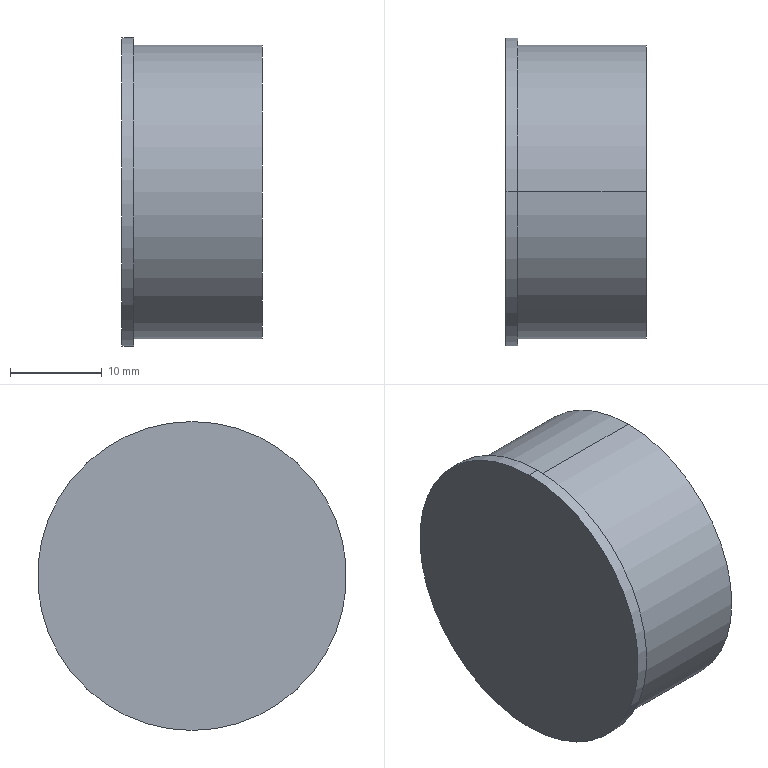Part | SolidWorks | features BaseBody 1 | 1 solid | 7 faces | box 15.3 x 33.7 x 33.7 mm | volume 12419 mm3 | cylinder 4 | plane 3 | commonest cylinder face diameters 32 x2 33.7 x2
STEP:
#1=CARTESIAN_POINT('',(209.5,-84.,161.471));
#2=VERTEX_POINT('',#1);
#3=CARTESIAN_POINT('',(209.5,-84.,127.771));
#4=VERTEX_POINT('',#3);
#5=CARTESIAN_POINT('',(209.5,-84.,144.621));
#6=DIRECTION('',(-1.,0.,0.));
#7=DIRECTION('',(0.,0.,1.));
#8=AXIS2_PLACEMENT_3D('',#5,#6,#7);
#9=CIRCLE('',#8,16.85);
#10=EDGE_CURVE('',#2,#4,#9,.T.);
#11=ORIENTED_EDGE('',*,*,#10,.T.);
#12=CARTESIAN_POINT('',(208.2,-84.,127.771));
#13=VERTEX_POINT('',#12);
#14=CARTESIAN_POINT('',(209.5,-84.,127.771));
#15=DIRECTION('',(-1.,0.,0.));
#16=VECTOR('',#15,1000.);
#17=LINE('',#14,#16);
#18=EDGE_CURVE('',#4,#13,#17,.T.);
#19=ORIENTED_EDGE('',*,*,#18,.T.);
#20=CARTESIAN_POINT('',(208.2,-84.,161.471));
#21=VERTEX_POINT('',#20);
#22=CARTESIAN_POINT('',(208.2,-84.,144.621));
#23=DIRECTION('',(1.,0.,0.));
#24=DIRECTION('',(0.,0.,1.));
#25=AXIS2_PLACEMENT_3D('',#22,#23,#24);
#26=CIRCLE('',#25,16.85);
#27=EDGE_CURVE('',#13,#21,#26,.T.);
#28=ORIENTED_EDGE('',*,*,#27,.T.);
#29=CARTESIAN_POINT('',(209.5,-84.,161.471));
#30=DIRECTION('',(-1.,0.,0.));
#31=VECTOR('',#30,1000.);
#32=LINE('',#29,#31);
#33=EDGE_CURVE('',#2,#21,#32,.T.);
#34=ORIENTED_EDGE('',*,*,#33,.F.);
#35=EDGE_LOOP('',(#11,#19,#28,#34));
#36=FACE_OUTER_BOUND('',#35,.T.);
#37=CARTESIAN_POINT('',(209.5,-84.,144.621));
#38=DIRECTION('',(-1.,0.,0.));
#39=DIRECTION('',(0.,0.,1.));
#40=AXIS2_PLACEMENT_3D('',#37,#38,#39);
#41=CYLINDRICAL_SURFACE('',#40,16.85);
#42=ADVANCED_FACE('',(#36),#41,.T.);
#43=CARTESIAN_POINT('',(223.5,-84.,160.621));
#44=VERTEX_POINT('',#43);
#45=CARTESIAN_POINT('',(223.5,-84.,128.621));
#46=VERTEX_POINT('',#45);
#47=CARTESIAN_POINT('',(223.5,-84.,144.621));
#48=DIRECTION('',(-1.,0.,0.));
#49=DIRECTION('',(0.,0.,1.));
#50=AXIS2_PLACEMENT_3D('',#47,#48,#49);
#51=CIRCLE('',#50,16.);
#52=EDGE_CURVE('',#44,#46,#51,.T.);
#53=ORIENTED_EDGE('',*,*,#52,.T.);
#54=CARTESIAN_POINT('',(209.5,-84.,128.621));
#55=VERTEX_POINT('',#54);
#56=CARTESIAN_POINT('',(223.5,-84.,128.621));
#57=DIRECTION('',(-1.,0.,0.));
#58=VECTOR('',#57,1000.);
#59=LINE('',#56,#58);
#60=EDGE_CURVE('',#46,#55,#59,.T.);
#61=ORIENTED_EDGE('',*,*,#60,.T.);
#62=CARTESIAN_POINT('',(209.5,-84.,160.621));
#63=VERTEX_POINT('',#62);
#64=CARTESIAN_POINT('',(209.5,-84.,144.621));
#65=DIRECTION('',(-1.,0.,0.));
#66=DIRECTION('',(0.,0.,1.));
#67=AXIS2_PLACEMENT_3D('',#64,#65,#66);
#68=CIRCLE('',#67,16.);
#69=EDGE_CURVE('',#63,#55,#68,.T.);
#70=ORIENTED_EDGE('',*,*,#69,.F.);
#71=CARTESIAN_POINT('',(223.5,-84.,160.621));
#72=DIRECTION('',(-1.,0.,0.));
#73=VECTOR('',#72,1000.);
#74=LINE('',#71,#73);
#75=EDGE_CURVE('',#44,#63,#74,.T.);
#76=ORIENTED_EDGE('',*,*,#75,.F.);
#77=EDGE_LOOP('',(#53,#61,#70,#76));
#78=FACE_OUTER_BOUND('',#77,.T.);
#79=CARTESIAN_POINT('',(223.5,-84.,144.621));
#80=DIRECTION('',(-1.,0.,0.));
#81=DIRECTION('',(0.,0.,1.));
#82=AXIS2_PLACEMENT_3D('',#79,#80,#81);
#83=CYLINDRICAL_SURFACE('',#82,16.);
#84=ADVANCED_FACE('',(#78),#83,.T.);
#85=CARTESIAN_POINT('',(208.2,-84.,144.621));
#86=DIRECTION('',(1.,0.,0.));
#87=DIRECTION('',(0.,0.,1.));
#88=AXIS2_PLACEMENT_3D('',#85,#86,#87);
#89=CIRCLE('',#88,16.85);
#90=EDGE_CURVE('',#21,#13,#89,.T.);
#91=ORIENTED_EDGE('',*,*,#90,.F.);
#92=ORIENTED_EDGE('',*,*,#27,.F.);
#93=EDGE_LOOP('',(#91,#92));
#94=FACE_OUTER_BOUND('',#93,.T.);
#95=CARTESIAN_POINT('',(208.2,-84.,144.621));
#96=DIRECTION('',(1.,0.,0.));
#97=DIRECTION('',(0.,0.,-1.));
#98=AXIS2_PLACEMENT_3D('',#95,#96,#97);
#99=PLANE('',#98);
#100=ADVANCED_FACE('',(#94),#99,.F.);
#101=ORIENTED_EDGE('',*,*,#18,.F.);
#102=CARTESIAN_POINT('',(209.5,-84.,144.621));
#103=DIRECTION('',(-1.,0.,0.));
#104=DIRECTION('',(0.,0.,1.));
#105=AXIS2_PLACEMENT_3D('',#102,#103,#104);
#106=CIRCLE('',#105,16.85);
#107=EDGE_CURVE('',#4,#2,#106,.T.);
#108=ORIENTED_EDGE('',*,*,#107,.T.);
#109=ORIENTED_EDGE('',*,*,#33,.T.);
#110=ORIENTED_EDGE('',*,*,#90,.T.);
#111=EDGE_LOOP('',(#101,#108,#109,#110));
#112=FACE_OUTER_BOUND('',#111,.T.);
#113=CARTESIAN_POINT('',(209.5,-84.,144.621));
#114=DIRECTION('',(-1.,0.,0.));
#115=DIRECTION('',(0.,0.,1.));
#116=AXIS2_PLACEMENT_3D('',#113,#114,#115);
#117=CYLINDRICAL_SURFACE('',#116,16.85);
#118=ADVANCED_FACE('',(#112),#117,.T.);
#119=ORIENTED_EDGE('',*,*,#69,.T.);
#120=CARTESIAN_POINT('',(209.5,-84.,144.621));
#121=DIRECTION('',(-1.,0.,0.));
#122=DIRECTION('',(0.,0.,1.));
#123=AXIS2_PLACEMENT_3D('',#120,#121,#122);
#124=CIRCLE('',#123,16.);
#125=EDGE_CURVE('',#55,#63,#124,.T.);
#126=ORIENTED_EDGE('',*,*,#125,.T.);
#127=EDGE_LOOP('',(#119,#126));
#128=FACE_BOUND('',#127,.T.);
#129=ORIENTED_EDGE('',*,*,#10,.F.);
#130=ORIENTED_EDGE('',*,*,#107,.F.);
#131=EDGE_LOOP('',(#129,#130));
#132=FACE_OUTER_BOUND('',#131,.T.);
#133=CARTESIAN_POINT('',(209.5,-84.,144.621));
#134=DIRECTION('',(1.,0.,0.));
#135=DIRECTION('',(0.,0.,-1.));
#136=AXIS2_PLACEMENT_3D('',#133,#134,#135);
#137=PLANE('',#136);
#138=ADVANCED_FACE('',(#128,#132),#137,.T.);
#139=ORIENTED_EDGE('',*,*,#60,.F.);
#140=CARTESIAN_POINT('',(223.5,-84.,144.621));
#141=DIRECTION('',(-1.,0.,0.));
#142=DIRECTION('',(0.,0.,1.));
#143=AXIS2_PLACEMENT_3D('',#140,#141,#142);
#144=CIRCLE('',#143,16.);
#145=EDGE_CURVE('',#46,#44,#144,.T.);
#146=ORIENTED_EDGE('',*,*,#145,.T.);
#147=ORIENTED_EDGE('',*,*,#75,.T.);
#148=ORIENTED_EDGE('',*,*,#125,.F.);
#149=EDGE_LOOP('',(#139,#146,#147,#148));
#150=FACE_OUTER_BOUND('',#149,.T.);
#151=CARTESIAN_POINT('',(223.5,-84.,144.621));
#152=DIRECTION('',(-1.,0.,0.));
#153=DIRECTION('',(0.,0.,1.));
#154=AXIS2_PLACEMENT_3D('',#151,#152,#153);
#155=CYLINDRICAL_SURFACE('',#154,16.);
#156=ADVANCED_FACE('',(#150),#155,.T.);
#157=ORIENTED_EDGE('',*,*,#52,.F.);
#158=ORIENTED_EDGE('',*,*,#145,.F.);
#159=EDGE_LOOP('',(#157,#158));
#160=FACE_OUTER_BOUND('',#159,.T.);
#161=CARTESIAN_POINT('',(223.5,-84.,144.621));
#162=DIRECTION('',(1.,0.,0.));
#163=DIRECTION('',(0.,0.,-1.));
#164=AXIS2_PLACEMENT_3D('',#161,#162,#163);
#165=PLANE('',#164);
#166=ADVANCED_FACE('',(#160),#165,.T.);
#167=CLOSED_SHELL('',(#42,#84,#100,#118,#138,#156,#166));
#168=MANIFOLD_SOLID_BREP('',#167);
#169=CARTESIAN_POINT('',(0.,0.,0.));
#170=DIRECTION('',(0.,0.,1.));
#171=DIRECTION('',(1.,0.,0.));
#172=AXIS2_PLACEMENT_3D('',#169,#170,#171);
#173=(LENGTH_UNIT()NAMED_UNIT(*)SI_UNIT(.MILLI.,.METRE.));
#174=UNCERTAINTY_MEASURE_WITH_UNIT(LENGTH_MEASURE(0.00001),#173,'','');
#175=(NAMED_UNIT(*)PLANE_ANGLE_UNIT()SI_UNIT($,.RADIAN.));
#176=(NAMED_UNIT(*)SI_UNIT($,.STERADIAN.)SOLID_ANGLE_UNIT());
#177=(GEOMETRIC_REPRESENTATION_CONTEXT(3)GLOBAL_UNCERTAINTY_ASSIGNED_CONTEXT((#174))GLOBAL_UNIT_ASSIGNED_CONTEXT((#173,#175,#176))REPRESENTATION_CONTEXT('',''));
#178=ADVANCED_BREP_SHAPE_REPRESENTATION('',(#168,#172),#177);